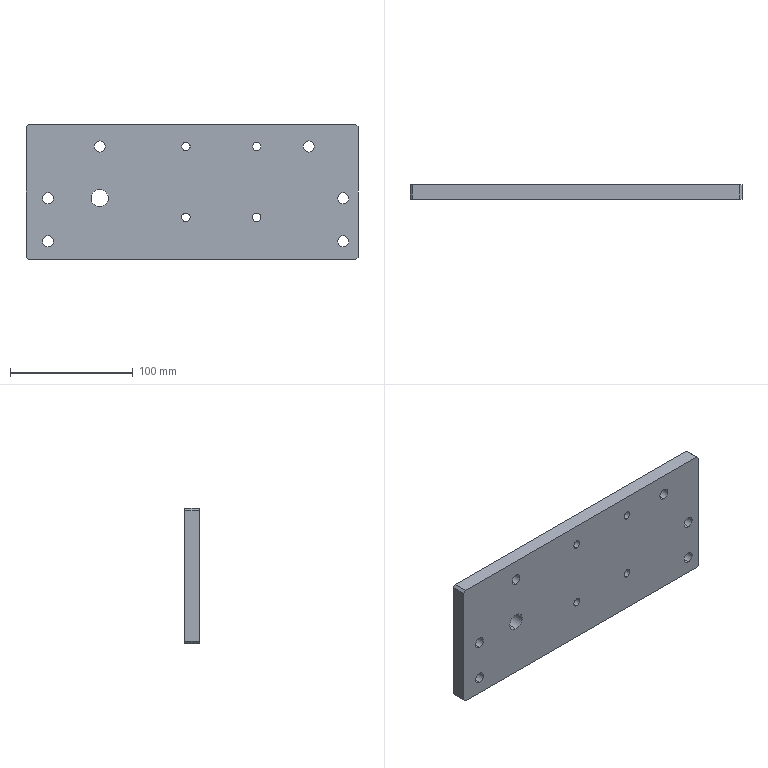Part | STEP file | 1 solid | 32 faces | box 270 x 12 x 110 mm | volume 348133 mm3 | cylinder 22 | plane 10 | commonest cylinder face diameters 9 x12 6.8 x8 14 x2